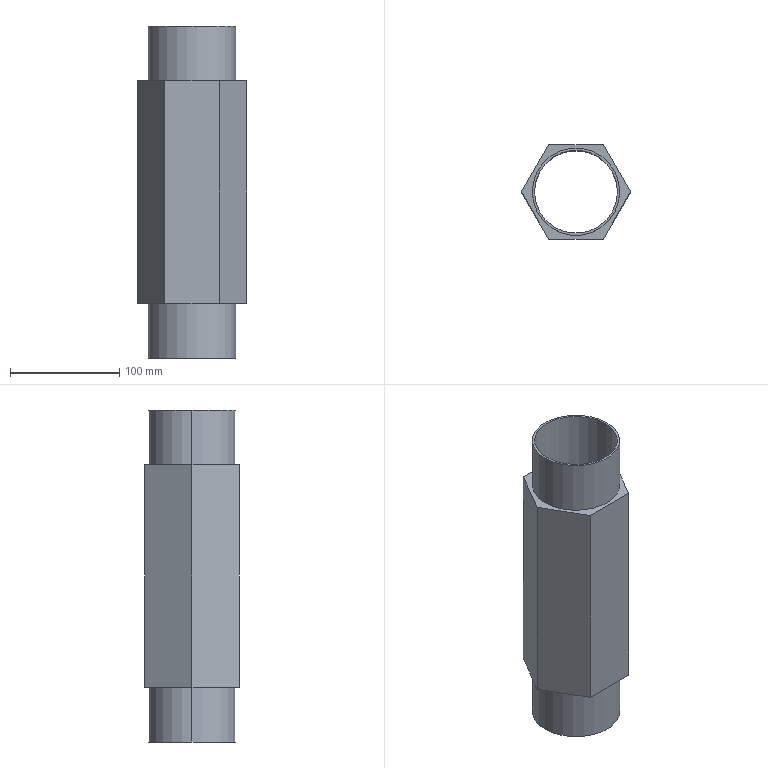Part | SolidWorks | features BaseBody 1 | 1 solid | 16 faces | box 100 x 86.603 x 304 mm | volume 448590 mm3 | plane 10 | cylinder 6 | commonest cylinder face diameters 80 x4 76 x2
STEP:
#1=CARTESIAN_POINT('',(38.,0.,50.));
#2=VERTEX_POINT('',#1);
#3=CARTESIAN_POINT('',(-38.,0.,50.));
#4=VERTEX_POINT('',#3);
#5=CARTESIAN_POINT('',(0.,0.,50.));
#6=DIRECTION('',(0.,0.,-1.));
#7=DIRECTION('',(1.,0.,0.));
#8=AXIS2_PLACEMENT_3D('',#5,#6,#7);
#9=CIRCLE('',#8,38.);
#10=EDGE_CURVE('',#2,#4,#9,.T.);
#11=ORIENTED_EDGE('',*,*,#10,.F.);
#12=CARTESIAN_POINT('',(38.,0.,-254.));
#13=VERTEX_POINT('',#12);
#14=CARTESIAN_POINT('',(38.,0.,100.));
#15=DIRECTION('',(0.,0.,-1.));
#16=VECTOR('',#15,1000.);
#17=LINE('',#14,#16);
#18=EDGE_CURVE('',#2,#13,#17,.T.);
#19=ORIENTED_EDGE('',*,*,#18,.T.);
#20=CARTESIAN_POINT('',(-38.,0.,-254.));
#21=VERTEX_POINT('',#20);
#22=CARTESIAN_POINT('',(0.,0.,-254.));
#23=DIRECTION('',(0.,0.,-1.));
#24=DIRECTION('',(1.,0.,0.));
#25=AXIS2_PLACEMENT_3D('',#22,#23,#24);
#26=CIRCLE('',#25,38.);
#27=EDGE_CURVE('',#13,#21,#26,.T.);
#28=ORIENTED_EDGE('',*,*,#27,.T.);
#29=CARTESIAN_POINT('',(-38.,0.,100.));
#30=DIRECTION('',(0.,0.,-1.));
#31=VECTOR('',#30,1000.);
#32=LINE('',#29,#31);
#33=EDGE_CURVE('',#4,#21,#32,.T.);
#34=ORIENTED_EDGE('',*,*,#33,.F.);
#35=EDGE_LOOP('',(#11,#19,#28,#34));
#36=FACE_OUTER_BOUND('',#35,.T.);
#37=CARTESIAN_POINT('',(0.,0.,100.));
#38=DIRECTION('',(0.,0.,-1.));
#39=DIRECTION('',(-1.,0.,0.));
#40=AXIS2_PLACEMENT_3D('',#37,#38,#39);
#41=CYLINDRICAL_SURFACE('',#40,38.);
#42=ADVANCED_FACE('',(#36),#41,.F.);
#43=CARTESIAN_POINT('',(40.,0.,50.));
#44=VERTEX_POINT('',#43);
#45=CARTESIAN_POINT('',(-40.,0.,50.));
#46=VERTEX_POINT('',#45);
#47=CARTESIAN_POINT('',(0.,0.,50.));
#48=DIRECTION('',(0.,0.,1.));
#49=DIRECTION('',(1.,0.,0.));
#50=AXIS2_PLACEMENT_3D('',#47,#48,#49);
#51=CIRCLE('',#50,40.);
#52=EDGE_CURVE('',#44,#46,#51,.T.);
#53=ORIENTED_EDGE('',*,*,#52,.F.);
#54=CARTESIAN_POINT('',(40.,0.,0.));
#55=VERTEX_POINT('',#54);
#56=CARTESIAN_POINT('',(40.,0.,50.));
#57=DIRECTION('',(0.,0.,-1.));
#58=VECTOR('',#57,1000.);
#59=LINE('',#56,#58);
#60=EDGE_CURVE('',#44,#55,#59,.T.);
#61=ORIENTED_EDGE('',*,*,#60,.T.);
#62=CARTESIAN_POINT('',(-40.,0.,0.));
#63=VERTEX_POINT('',#62);
#64=CARTESIAN_POINT('',(0.,0.,0.));
#65=DIRECTION('',(0.,0.,-1.));
#66=DIRECTION('',(1.,0.,0.));
#67=AXIS2_PLACEMENT_3D('',#64,#65,#66);
#68=CIRCLE('',#67,40.);
#69=EDGE_CURVE('',#63,#55,#68,.T.);
#70=ORIENTED_EDGE('',*,*,#69,.F.);
#71=CARTESIAN_POINT('',(-40.,0.,50.));
#72=DIRECTION('',(0.,0.,-1.));
#73=VECTOR('',#72,1000.);
#74=LINE('',#71,#73);
#75=EDGE_CURVE('',#46,#63,#74,.T.);
#76=ORIENTED_EDGE('',*,*,#75,.F.);
#77=EDGE_LOOP('',(#53,#61,#70,#76));
#78=FACE_OUTER_BOUND('',#77,.T.);
#79=CARTESIAN_POINT('',(0.,0.,50.));
#80=DIRECTION('',(0.,0.,-1.));
#81=DIRECTION('',(-1.,0.,0.));
#82=AXIS2_PLACEMENT_3D('',#79,#80,#81);
#83=CYLINDRICAL_SURFACE('',#82,40.);
#84=ADVANCED_FACE('',(#78),#83,.T.);
#85=CARTESIAN_POINT('',(-40.,0.,-204.));
#86=VERTEX_POINT('',#85);
#87=CARTESIAN_POINT('',(40.,0.,-204.));
#88=VERTEX_POINT('',#87);
#89=CARTESIAN_POINT('',(0.,0.,-204.));
#90=DIRECTION('',(0.,0.,-1.));
#91=DIRECTION('',(1.,0.,0.));
#92=AXIS2_PLACEMENT_3D('',#89,#90,#91);
#93=CIRCLE('',#92,40.);
#94=EDGE_CURVE('',#86,#88,#93,.T.);
#95=ORIENTED_EDGE('',*,*,#94,.T.);
#96=CARTESIAN_POINT('',(40.,0.,-254.));
#97=VERTEX_POINT('',#96);
#98=CARTESIAN_POINT('',(40.,0.,50.));
#99=DIRECTION('',(0.,0.,-1.));
#100=VECTOR('',#99,1000.);
#101=LINE('',#98,#100);
#102=EDGE_CURVE('',#88,#97,#101,.T.);
#103=ORIENTED_EDGE('',*,*,#102,.T.);
#104=CARTESIAN_POINT('',(-40.,0.,-254.));
#105=VERTEX_POINT('',#104);
#106=CARTESIAN_POINT('',(0.,0.,-254.));
#107=DIRECTION('',(0.,0.,1.));
#108=DIRECTION('',(1.,0.,0.));
#109=AXIS2_PLACEMENT_3D('',#106,#107,#108);
#110=CIRCLE('',#109,40.);
#111=EDGE_CURVE('',#97,#105,#110,.T.);
#112=ORIENTED_EDGE('',*,*,#111,.T.);
#113=CARTESIAN_POINT('',(-40.,0.,50.));
#114=DIRECTION('',(0.,0.,-1.));
#115=VECTOR('',#114,1000.);
#116=LINE('',#113,#115);
#117=EDGE_CURVE('',#86,#105,#116,.T.);
#118=ORIENTED_EDGE('',*,*,#117,.F.);
#119=EDGE_LOOP('',(#95,#103,#112,#118));
#120=FACE_OUTER_BOUND('',#119,.T.);
#121=CARTESIAN_POINT('',(0.,0.,50.));
#122=DIRECTION('',(0.,0.,-1.));
#123=DIRECTION('',(-1.,0.,0.));
#124=AXIS2_PLACEMENT_3D('',#121,#122,#123);
#125=CYLINDRICAL_SURFACE('',#124,40.);
#126=ADVANCED_FACE('',(#120),#125,.T.);
#127=CARTESIAN_POINT('',(-50.,0.,-204.));
#128=VERTEX_POINT('',#127);
#129=CARTESIAN_POINT('',(-25.,-43.301,-204.));
#130=VERTEX_POINT('',#129);
#131=CARTESIAN_POINT('',(-50.,0.,-204.));
#132=DIRECTION('',(0.5,-0.866,0.));
#133=VECTOR('',#132,1000.);
#134=LINE('',#131,#133);
#135=EDGE_CURVE('',#128,#130,#134,.T.);
#136=ORIENTED_EDGE('',*,*,#135,.T.);
#137=CARTESIAN_POINT('',(-25.,-43.301,0.));
#138=VERTEX_POINT('',#137);
#139=CARTESIAN_POINT('',(-25.,-43.301,0.));
#140=DIRECTION('',(0.,0.,-1.));
#141=VECTOR('',#140,1000.);
#142=LINE('',#139,#141);
#143=EDGE_CURVE('',#138,#130,#142,.T.);
#144=ORIENTED_EDGE('',*,*,#143,.F.);
#145=CARTESIAN_POINT('',(-50.,0.,0.));
#146=VERTEX_POINT('',#145);
#147=CARTESIAN_POINT('',(-50.,0.,0.));
#148=DIRECTION('',(0.5,-0.866,0.));
#149=VECTOR('',#148,1000.);
#150=LINE('',#147,#149);
#151=EDGE_CURVE('',#146,#138,#150,.T.);
#152=ORIENTED_EDGE('',*,*,#151,.F.);
#153=CARTESIAN_POINT('',(-50.,0.,0.));
#154=DIRECTION('',(0.,0.,-1.));
#155=VECTOR('',#154,1000.);
#156=LINE('',#153,#155);
#157=EDGE_CURVE('',#146,#128,#156,.T.);
#158=ORIENTED_EDGE('',*,*,#157,.T.);
#159=EDGE_LOOP('',(#136,#144,#152,#158));
#160=FACE_OUTER_BOUND('',#159,.T.);
#161=CARTESIAN_POINT('',(-50.,0.,0.));
#162=DIRECTION('',(0.866,0.5,0.));
#163=DIRECTION('',(-0.5,0.866,0.));
#164=AXIS2_PLACEMENT_3D('',#161,#162,#163);
#165=PLANE('',#164);
#166=ADVANCED_FACE('',(#160),#165,.F.);
#167=CARTESIAN_POINT('',(25.,-43.301,-204.));
#168=VERTEX_POINT('',#167);
#169=CARTESIAN_POINT('',(-25.,-43.301,-204.));
#170=DIRECTION('',(1.,0.,0.));
#171=VECTOR('',#170,1000.);
#172=LINE('',#169,#171);
#173=EDGE_CURVE('',#130,#168,#172,.T.);
#174=ORIENTED_EDGE('',*,*,#173,.T.);
#175=CARTESIAN_POINT('',(25.,-43.301,0.));
#176=VERTEX_POINT('',#175);
#177=CARTESIAN_POINT('',(25.,-43.301,0.));
#178=DIRECTION('',(0.,0.,-1.));
#179=VECTOR('',#178,1000.);
#180=LINE('',#177,#179);
#181=EDGE_CURVE('',#176,#168,#180,.T.);
#182=ORIENTED_EDGE('',*,*,#181,.F.);
#183=CARTESIAN_POINT('',(-25.,-43.301,0.));
#184=DIRECTION('',(1.,0.,0.));
#185=VECTOR('',#184,1000.);
#186=LINE('',#183,#185);
#187=EDGE_CURVE('',#138,#176,#186,.T.);
#188=ORIENTED_EDGE('',*,*,#187,.F.);
#189=ORIENTED_EDGE('',*,*,#143,.T.);
#190=EDGE_LOOP('',(#174,#182,#188,#189));
#191=FACE_OUTER_BOUND('',#190,.T.);
#192=CARTESIAN_POINT('',(-25.,-43.301,0.));
#193=DIRECTION('',(0.,1.,0.));
#194=DIRECTION('',(-1.,0.,0.));
#195=AXIS2_PLACEMENT_3D('',#192,#193,#194);
#196=PLANE('',#195);
#197=ADVANCED_FACE('',(#191),#196,.F.);
#198=CARTESIAN_POINT('',(50.,0.,-204.));
#199=VERTEX_POINT('',#198);
#200=CARTESIAN_POINT('',(25.,-43.301,-204.));
#201=DIRECTION('',(0.5,0.866,0.));
#202=VECTOR('',#201,1000.);
#203=LINE('',#200,#202);
#204=EDGE_CURVE('',#168,#199,#203,.T.);
#205=ORIENTED_EDGE('',*,*,#204,.T.);
#206=CARTESIAN_POINT('',(50.,0.,0.));
#207=VERTEX_POINT('',#206);
#208=CARTESIAN_POINT('',(50.,0.,0.));
#209=DIRECTION('',(0.,0.,-1.));
#210=VECTOR('',#209,1000.);
#211=LINE('',#208,#210);
#212=EDGE_CURVE('',#207,#199,#211,.T.);
#213=ORIENTED_EDGE('',*,*,#212,.F.);
#214=CARTESIAN_POINT('',(25.,-43.301,0.));
#215=DIRECTION('',(0.5,0.866,0.));
#216=VECTOR('',#215,1000.);
#217=LINE('',#214,#216);
#218=EDGE_CURVE('',#176,#207,#217,.T.);
#219=ORIENTED_EDGE('',*,*,#218,.F.);
#220=ORIENTED_EDGE('',*,*,#181,.T.);
#221=EDGE_LOOP('',(#205,#213,#219,#220));
#222=FACE_OUTER_BOUND('',#221,.T.);
#223=CARTESIAN_POINT('',(25.,-43.301,0.));
#224=DIRECTION('',(-0.866,0.5,0.));
#225=DIRECTION('',(-0.5,-0.866,0.));
#226=AXIS2_PLACEMENT_3D('',#223,#224,#225);
#227=PLANE('',#226);
#228=ADVANCED_FACE('',(#222),#227,.F.);
#229=CARTESIAN_POINT('',(25.,43.301,-204.));
#230=VERTEX_POINT('',#229);
#231=CARTESIAN_POINT('',(50.,0.,-204.));
#232=DIRECTION('',(-0.5,0.866,0.));
#233=VECTOR('',#232,1000.);
#234=LINE('',#231,#233);
#235=EDGE_CURVE('',#199,#230,#234,.T.);
#236=ORIENTED_EDGE('',*,*,#235,.T.);
#237=CARTESIAN_POINT('',(25.,43.301,0.));
#238=VERTEX_POINT('',#237);
#239=CARTESIAN_POINT('',(25.,43.301,0.));
#240=DIRECTION('',(0.,0.,-1.));
#241=VECTOR('',#240,1000.);
#242=LINE('',#239,#241);
#243=EDGE_CURVE('',#238,#230,#242,.T.);
#244=ORIENTED_EDGE('',*,*,#243,.F.);
#245=CARTESIAN_POINT('',(50.,0.,0.));
#246=DIRECTION('',(-0.5,0.866,0.));
#247=VECTOR('',#246,1000.);
#248=LINE('',#245,#247);
#249=EDGE_CURVE('',#207,#238,#248,.T.);
#250=ORIENTED_EDGE('',*,*,#249,.F.);
#251=ORIENTED_EDGE('',*,*,#212,.T.);
#252=EDGE_LOOP('',(#236,#244,#250,#251));
#253=FACE_OUTER_BOUND('',#252,.T.);
#254=CARTESIAN_POINT('',(50.,0.,0.));
#255=DIRECTION('',(-0.866,-0.5,0.));
#256=DIRECTION('',(0.5,-0.866,0.));
#257=AXIS2_PLACEMENT_3D('',#254,#255,#256);
#258=PLANE('',#257);
#259=ADVANCED_FACE('',(#253),#258,.F.);
#260=CARTESIAN_POINT('',(-25.,43.301,-204.));
#261=VERTEX_POINT('',#260);
#262=CARTESIAN_POINT('',(25.,43.301,-204.));
#263=DIRECTION('',(-1.,0.,0.));
#264=VECTOR('',#263,1000.);
#265=LINE('',#262,#264);
#266=EDGE_CURVE('',#230,#261,#265,.T.);
#267=ORIENTED_EDGE('',*,*,#266,.T.);
#268=CARTESIAN_POINT('',(-25.,43.301,0.));
#269=VERTEX_POINT('',#268);
#270=CARTESIAN_POINT('',(-25.,43.301,0.));
#271=DIRECTION('',(0.,0.,-1.));
#272=VECTOR('',#271,1000.);
#273=LINE('',#270,#272);
#274=EDGE_CURVE('',#269,#261,#273,.T.);
#275=ORIENTED_EDGE('',*,*,#274,.F.);
#276=CARTESIAN_POINT('',(25.,43.301,0.));
#277=DIRECTION('',(-1.,0.,0.));
#278=VECTOR('',#277,1000.);
#279=LINE('',#276,#278);
#280=EDGE_CURVE('',#238,#269,#279,.T.);
#281=ORIENTED_EDGE('',*,*,#280,.F.);
#282=ORIENTED_EDGE('',*,*,#243,.T.);
#283=EDGE_LOOP('',(#267,#275,#281,#282));
#284=FACE_OUTER_BOUND('',#283,.T.);
#285=CARTESIAN_POINT('',(25.,43.301,0.));
#286=DIRECTION('',(0.,-1.,0.));
#287=DIRECTION('',(1.,0.,0.));
#288=AXIS2_PLACEMENT_3D('',#285,#286,#287);
#289=PLANE('',#288);
#290=ADVANCED_FACE('',(#284),#289,.F.);
#291=CARTESIAN_POINT('',(-25.,43.301,-204.));
#292=DIRECTION('',(-0.5,-0.866,0.));
#293=VECTOR('',#292,1000.);
#294=LINE('',#291,#293);
#295=EDGE_CURVE('',#261,#128,#294,.T.);
#296=ORIENTED_EDGE('',*,*,#295,.T.);
#297=ORIENTED_EDGE('',*,*,#157,.F.);
#298=CARTESIAN_POINT('',(-25.,43.301,0.));
#299=DIRECTION('',(-0.5,-0.866,0.));
#300=VECTOR('',#299,1000.);
#301=LINE('',#298,#300);
#302=EDGE_CURVE('',#269,#146,#301,.T.);
#303=ORIENTED_EDGE('',*,*,#302,.F.);
#304=ORIENTED_EDGE('',*,*,#274,.T.);
#305=EDGE_LOOP('',(#296,#297,#303,#304));
#306=FACE_OUTER_BOUND('',#305,.T.);
#307=CARTESIAN_POINT('',(-25.,43.301,0.));
#308=DIRECTION('',(0.866,-0.5,0.));
#309=DIRECTION('',(0.5,0.866,0.));
#310=AXIS2_PLACEMENT_3D('',#307,#308,#309);
#311=PLANE('',#310);
#312=ADVANCED_FACE('',(#306),#311,.F.);
#313=ORIENTED_EDGE('',*,*,#69,.T.);
#314=CARTESIAN_POINT('',(0.,0.,0.));
#315=DIRECTION('',(0.,0.,-1.));
#316=DIRECTION('',(1.,0.,0.));
#317=AXIS2_PLACEMENT_3D('',#314,#315,#316);
#318=CIRCLE('',#317,40.);
#319=EDGE_CURVE('',#55,#63,#318,.T.);
#320=ORIENTED_EDGE('',*,*,#319,.T.);
#321=EDGE_LOOP('',(#313,#320));
#322=FACE_BOUND('',#321,.T.);
#323=ORIENTED_EDGE('',*,*,#151,.T.);
#324=ORIENTED_EDGE('',*,*,#187,.T.);
#325=ORIENTED_EDGE('',*,*,#218,.T.);
#326=ORIENTED_EDGE('',*,*,#249,.T.);
#327=ORIENTED_EDGE('',*,*,#280,.T.);
#328=ORIENTED_EDGE('',*,*,#302,.T.);
#329=EDGE_LOOP('',(#323,#324,#325,#326,#327,#328));
#330=FACE_OUTER_BOUND('',#329,.T.);
#331=CARTESIAN_POINT('',(0.,0.,0.));
#332=DIRECTION('',(0.,0.,1.));
#333=DIRECTION('',(1.,0.,0.));
#334=AXIS2_PLACEMENT_3D('',#331,#332,#333);
#335=PLANE('',#334);
#336=ADVANCED_FACE('',(#322,#330),#335,.T.);
#337=ORIENTED_EDGE('',*,*,#94,.F.);
#338=CARTESIAN_POINT('',(0.,0.,-204.));
#339=DIRECTION('',(0.,0.,-1.));
#340=DIRECTION('',(1.,0.,0.));
#341=AXIS2_PLACEMENT_3D('',#338,#339,#340);
#342=CIRCLE('',#341,40.);
#343=EDGE_CURVE('',#88,#86,#342,.T.);
#344=ORIENTED_EDGE('',*,*,#343,.F.);
#345=EDGE_LOOP('',(#337,#344));
#346=FACE_BOUND('',#345,.T.);
#347=ORIENTED_EDGE('',*,*,#135,.F.);
#348=ORIENTED_EDGE('',*,*,#295,.F.);
#349=ORIENTED_EDGE('',*,*,#266,.F.);
#350=ORIENTED_EDGE('',*,*,#235,.F.);
#351=ORIENTED_EDGE('',*,*,#204,.F.);
#352=ORIENTED_EDGE('',*,*,#173,.F.);
#353=EDGE_LOOP('',(#347,#348,#349,#350,#351,#352));
#354=FACE_OUTER_BOUND('',#353,.T.);
#355=CARTESIAN_POINT('',(0.,0.,-204.));
#356=DIRECTION('',(0.,0.,1.));
#357=DIRECTION('',(1.,0.,0.));
#358=AXIS2_PLACEMENT_3D('',#355,#356,#357);
#359=PLANE('',#358);
#360=ADVANCED_FACE('',(#346,#354),#359,.F.);
#361=CARTESIAN_POINT('',(0.,0.,-254.));
#362=DIRECTION('',(0.,0.,-1.));
#363=DIRECTION('',(1.,0.,0.));
#364=AXIS2_PLACEMENT_3D('',#361,#362,#363);
#365=CIRCLE('',#364,38.);
#366=EDGE_CURVE('',#21,#13,#365,.T.);
#367=ORIENTED_EDGE('',*,*,#366,.F.);
#368=ORIENTED_EDGE('',*,*,#27,.F.);
#369=EDGE_LOOP('',(#367,#368));
#370=FACE_BOUND('',#369,.T.);
#371=CARTESIAN_POINT('',(0.,0.,-254.));
#372=DIRECTION('',(0.,0.,1.));
#373=DIRECTION('',(1.,0.,0.));
#374=AXIS2_PLACEMENT_3D('',#371,#372,#373);
#375=CIRCLE('',#374,40.);
#376=EDGE_CURVE('',#105,#97,#375,.T.);
#377=ORIENTED_EDGE('',*,*,#376,.F.);
#378=ORIENTED_EDGE('',*,*,#111,.F.);
#379=EDGE_LOOP('',(#377,#378));
#380=FACE_OUTER_BOUND('',#379,.T.);
#381=CARTESIAN_POINT('',(0.,0.,-254.));
#382=DIRECTION('',(0.,0.,1.));
#383=DIRECTION('',(1.,0.,0.));
#384=AXIS2_PLACEMENT_3D('',#381,#382,#383);
#385=PLANE('',#384);
#386=ADVANCED_FACE('',(#370,#380),#385,.F.);
#387=ORIENTED_EDGE('',*,*,#102,.F.);
#388=ORIENTED_EDGE('',*,*,#343,.T.);
#389=ORIENTED_EDGE('',*,*,#117,.T.);
#390=ORIENTED_EDGE('',*,*,#376,.T.);
#391=EDGE_LOOP('',(#387,#388,#389,#390));
#392=FACE_OUTER_BOUND('',#391,.T.);
#393=CARTESIAN_POINT('',(0.,0.,50.));
#394=DIRECTION('',(0.,0.,-1.));
#395=DIRECTION('',(-1.,0.,0.));
#396=AXIS2_PLACEMENT_3D('',#393,#394,#395);
#397=CYLINDRICAL_SURFACE('',#396,40.);
#398=ADVANCED_FACE('',(#392),#397,.T.);
#399=ORIENTED_EDGE('',*,*,#60,.F.);
#400=CARTESIAN_POINT('',(0.,0.,50.));
#401=DIRECTION('',(0.,0.,1.));
#402=DIRECTION('',(1.,0.,0.));
#403=AXIS2_PLACEMENT_3D('',#400,#401,#402);
#404=CIRCLE('',#403,40.);
#405=EDGE_CURVE('',#46,#44,#404,.T.);
#406=ORIENTED_EDGE('',*,*,#405,.F.);
#407=ORIENTED_EDGE('',*,*,#75,.T.);
#408=ORIENTED_EDGE('',*,*,#319,.F.);
#409=EDGE_LOOP('',(#399,#406,#407,#408));
#410=FACE_OUTER_BOUND('',#409,.T.);
#411=CARTESIAN_POINT('',(0.,0.,50.));
#412=DIRECTION('',(0.,0.,-1.));
#413=DIRECTION('',(-1.,0.,0.));
#414=AXIS2_PLACEMENT_3D('',#411,#412,#413);
#415=CYLINDRICAL_SURFACE('',#414,40.);
#416=ADVANCED_FACE('',(#410),#415,.T.);
#417=CARTESIAN_POINT('',(0.,0.,50.));
#418=DIRECTION('',(0.,0.,-1.));
#419=DIRECTION('',(1.,0.,0.));
#420=AXIS2_PLACEMENT_3D('',#417,#418,#419);
#421=CIRCLE('',#420,38.);
#422=EDGE_CURVE('',#4,#2,#421,.T.);
#423=ORIENTED_EDGE('',*,*,#422,.T.);
#424=ORIENTED_EDGE('',*,*,#10,.T.);
#425=EDGE_LOOP('',(#423,#424));
#426=FACE_BOUND('',#425,.T.);
#427=ORIENTED_EDGE('',*,*,#405,.T.);
#428=ORIENTED_EDGE('',*,*,#52,.T.);
#429=EDGE_LOOP('',(#427,#428));
#430=FACE_OUTER_BOUND('',#429,.T.);
#431=CARTESIAN_POINT('',(0.,0.,50.));
#432=DIRECTION('',(0.,0.,1.));
#433=DIRECTION('',(1.,0.,0.));
#434=AXIS2_PLACEMENT_3D('',#431,#432,#433);
#435=PLANE('',#434);
#436=ADVANCED_FACE('',(#426,#430),#435,.T.);
#437=ORIENTED_EDGE('',*,*,#18,.F.);
#438=ORIENTED_EDGE('',*,*,#422,.F.);
#439=ORIENTED_EDGE('',*,*,#33,.T.);
#440=ORIENTED_EDGE('',*,*,#366,.T.);
#441=EDGE_LOOP('',(#437,#438,#439,#440));
#442=FACE_OUTER_BOUND('',#441,.T.);
#443=CARTESIAN_POINT('',(0.,0.,100.));
#444=DIRECTION('',(0.,0.,-1.));
#445=DIRECTION('',(-1.,0.,0.));
#446=AXIS2_PLACEMENT_3D('',#443,#444,#445);
#447=CYLINDRICAL_SURFACE('',#446,38.);
#448=ADVANCED_FACE('',(#442),#447,.F.);
#449=CLOSED_SHELL('',(#42,#84,#126,#166,#197,#228,#259,#290,#312,#336,#360,#386,#398,#416,#436,#448));
#450=MANIFOLD_SOLID_BREP('',#449);
#451=CARTESIAN_POINT('',(0.,0.,0.));
#452=DIRECTION('',(0.,0.,1.));
#453=DIRECTION('',(1.,0.,0.));
#454=AXIS2_PLACEMENT_3D('',#451,#452,#453);
#455=(LENGTH_UNIT()NAMED_UNIT(*)SI_UNIT(.MILLI.,.METRE.));
#456=UNCERTAINTY_MEASURE_WITH_UNIT(LENGTH_MEASURE(0.00001),#455,'','');
#457=(NAMED_UNIT(*)PLANE_ANGLE_UNIT()SI_UNIT($,.RADIAN.));
#458=(NAMED_UNIT(*)SI_UNIT($,.STERADIAN.)SOLID_ANGLE_UNIT());
#459=(GEOMETRIC_REPRESENTATION_CONTEXT(3)GLOBAL_UNCERTAINTY_ASSIGNED_CONTEXT((#456))GLOBAL_UNIT_ASSIGNED_CONTEXT((#455,#457,#458))REPRESENTATION_CONTEXT('',''));
#460=ADVANCED_BREP_SHAPE_REPRESENTATION('',(#450,#454),#459);